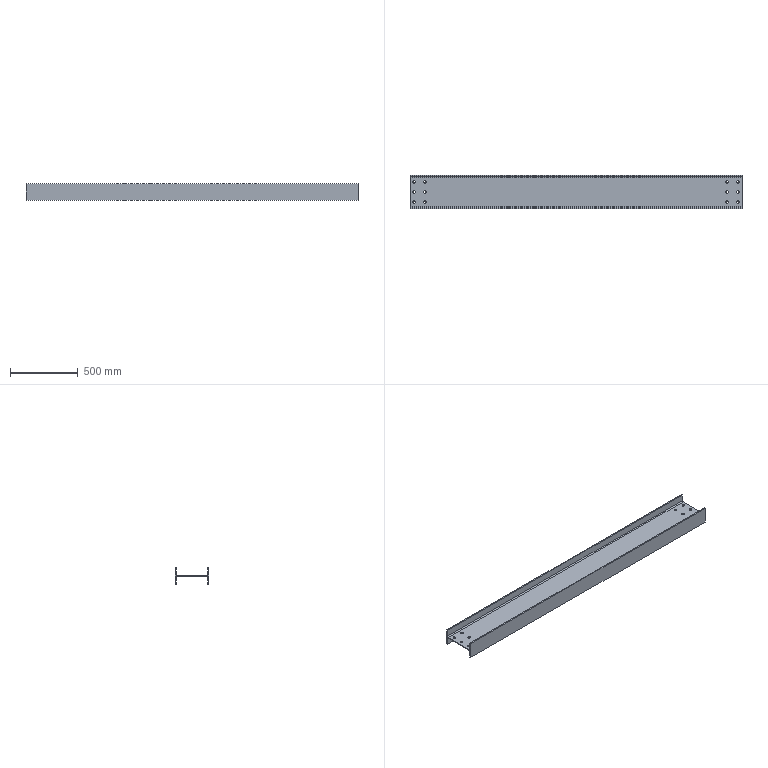Part | STEP file | 粉仓主梁8主体_Default<As Machined> | 1 solid | 42 faces | box 2455 x 250 x 125 mm | volume 9055569 mm3 | cylinder 28 | plane 14 | commonest cylinder face diameters 19 x24 16 x4